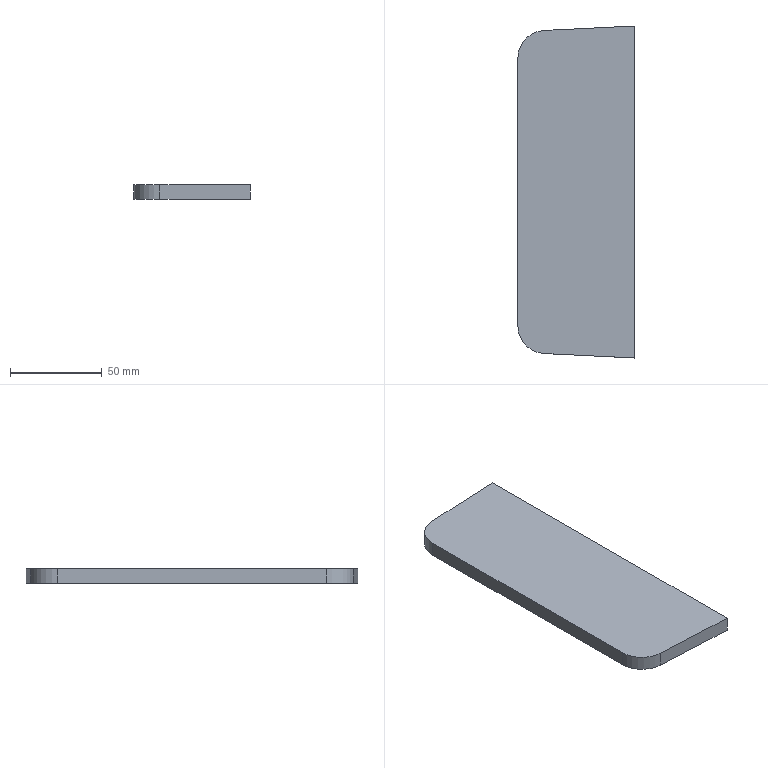Part | SolidWorks | features Extrusion 1 | 1 solid | 8 faces | box 63.5 x 181.351 x 8 mm | volume 89849 mm3 | plane 6 | cylinder 2 | commonest cylinder face diameters 30 x2
STEP:
#1=CARTESIAN_POINT('',(-31.75,-73.268,-4.));
#2=VERTEX_POINT('',#1);
#3=CARTESIAN_POINT('',(-17.488,-88.25,-4.));
#4=VERTEX_POINT('',#3);
#5=CARTESIAN_POINT('',(-16.75,-73.268,-4.));
#6=DIRECTION('',(0.,0.,1.));
#7=DIRECTION('',(1.,0.,0.));
#8=AXIS2_PLACEMENT_3D('',#5,#6,#7);
#9=CIRCLE('',#8,15.);
#10=EDGE_CURVE('',#2,#4,#9,.T.);
#11=ORIENTED_EDGE('',*,*,#10,.T.);
#12=CARTESIAN_POINT('',(-17.488,-88.25,4.));
#13=VERTEX_POINT('',#12);
#14=CARTESIAN_POINT('',(-17.488,-88.25,4.));
#15=DIRECTION('',(0.,0.,-1.));
#16=VECTOR('',#15,1000.);
#17=LINE('',#14,#16);
#18=EDGE_CURVE('',#13,#4,#17,.T.);
#19=ORIENTED_EDGE('',*,*,#18,.F.);
#20=CARTESIAN_POINT('',(-31.75,-73.268,4.));
#21=VERTEX_POINT('',#20);
#22=CARTESIAN_POINT('',(-16.75,-73.268,4.));
#23=DIRECTION('',(0.,0.,1.));
#24=DIRECTION('',(1.,0.,0.));
#25=AXIS2_PLACEMENT_3D('',#22,#23,#24);
#26=CIRCLE('',#25,15.);
#27=EDGE_CURVE('',#21,#13,#26,.T.);
#28=ORIENTED_EDGE('',*,*,#27,.F.);
#29=CARTESIAN_POINT('',(-31.75,-73.268,4.));
#30=DIRECTION('',(0.,0.,-1.));
#31=VECTOR('',#30,1000.);
#32=LINE('',#29,#31);
#33=EDGE_CURVE('',#21,#2,#32,.T.);
#34=ORIENTED_EDGE('',*,*,#33,.T.);
#35=EDGE_LOOP('',(#11,#19,#28,#34));
#36=FACE_OUTER_BOUND('',#35,.T.);
#37=CARTESIAN_POINT('',(-16.75,-73.268,4.));
#38=DIRECTION('',(0.,0.,-1.));
#39=DIRECTION('',(-1.,0.,0.));
#40=AXIS2_PLACEMENT_3D('',#37,#38,#39);
#41=CYLINDRICAL_SURFACE('',#40,15.);
#42=ADVANCED_FACE('',(#36),#41,.T.);
#43=CARTESIAN_POINT('',(31.75,-90.675,-4.));
#44=VERTEX_POINT('',#43);
#45=CARTESIAN_POINT('',(-17.488,-88.25,-4.));
#46=DIRECTION('',(0.9988,-0.0492,0.));
#47=VECTOR('',#46,1000.);
#48=LINE('',#45,#47);
#49=EDGE_CURVE('',#4,#44,#48,.T.);
#50=ORIENTED_EDGE('',*,*,#49,.T.);
#51=CARTESIAN_POINT('',(31.75,-90.675,4.));
#52=VERTEX_POINT('',#51);
#53=CARTESIAN_POINT('',(31.75,-90.675,4.));
#54=DIRECTION('',(0.,0.,-1.));
#55=VECTOR('',#54,1000.);
#56=LINE('',#53,#55);
#57=EDGE_CURVE('',#52,#44,#56,.T.);
#58=ORIENTED_EDGE('',*,*,#57,.F.);
#59=CARTESIAN_POINT('',(-17.488,-88.25,4.));
#60=DIRECTION('',(0.9988,-0.0492,0.));
#61=VECTOR('',#60,1000.);
#62=LINE('',#59,#61);
#63=EDGE_CURVE('',#13,#52,#62,.T.);
#64=ORIENTED_EDGE('',*,*,#63,.F.);
#65=ORIENTED_EDGE('',*,*,#18,.T.);
#66=EDGE_LOOP('',(#50,#58,#64,#65));
#67=FACE_OUTER_BOUND('',#66,.T.);
#68=CARTESIAN_POINT('',(-17.488,-88.25,4.));
#69=DIRECTION('',(0.0492,0.9988,0.));
#70=DIRECTION('',(-0.9988,0.0492,0.));
#71=AXIS2_PLACEMENT_3D('',#68,#69,#70);
#72=PLANE('',#71);
#73=ADVANCED_FACE('',(#67),#72,.F.);
#74=CARTESIAN_POINT('',(31.75,90.675,-4.));
#75=VERTEX_POINT('',#74);
#76=CARTESIAN_POINT('',(31.75,90.675,-4.));
#77=DIRECTION('',(0.,1.,0.));
#78=VECTOR('',#77,1000.);
#79=LINE('',#76,#78);
#80=EDGE_CURVE('',#44,#75,#79,.T.);
#81=ORIENTED_EDGE('',*,*,#80,.T.);
#82=CARTESIAN_POINT('',(31.75,90.675,4.));
#83=VERTEX_POINT('',#82);
#84=CARTESIAN_POINT('',(31.75,90.675,4.));
#85=DIRECTION('',(0.,0.,-1.));
#86=VECTOR('',#85,1000.);
#87=LINE('',#84,#86);
#88=EDGE_CURVE('',#83,#75,#87,.T.);
#89=ORIENTED_EDGE('',*,*,#88,.F.);
#90=CARTESIAN_POINT('',(31.75,90.675,4.));
#91=DIRECTION('',(0.,1.,0.));
#92=VECTOR('',#91,1000.);
#93=LINE('',#90,#92);
#94=EDGE_CURVE('',#52,#83,#93,.T.);
#95=ORIENTED_EDGE('',*,*,#94,.F.);
#96=ORIENTED_EDGE('',*,*,#57,.T.);
#97=EDGE_LOOP('',(#81,#89,#95,#96));
#98=FACE_OUTER_BOUND('',#97,.T.);
#99=CARTESIAN_POINT('',(31.75,90.675,4.));
#100=DIRECTION('',(-1.,0.,0.));
#101=DIRECTION('',(0.,0.,1.));
#102=AXIS2_PLACEMENT_3D('',#99,#100,#101);
#103=PLANE('',#102);
#104=ADVANCED_FACE('',(#98),#103,.F.);
#105=CARTESIAN_POINT('',(-17.488,88.25,-4.));
#106=VERTEX_POINT('',#105);
#107=CARTESIAN_POINT('',(-17.488,88.25,-4.));
#108=DIRECTION('',(-0.9988,-0.0492,0.));
#109=VECTOR('',#108,1000.);
#110=LINE('',#107,#109);
#111=EDGE_CURVE('',#75,#106,#110,.T.);
#112=ORIENTED_EDGE('',*,*,#111,.T.);
#113=CARTESIAN_POINT('',(-17.488,88.25,4.));
#114=VERTEX_POINT('',#113);
#115=CARTESIAN_POINT('',(-17.488,88.25,4.));
#116=DIRECTION('',(0.,0.,-1.));
#117=VECTOR('',#116,1000.);
#118=LINE('',#115,#117);
#119=EDGE_CURVE('',#114,#106,#118,.T.);
#120=ORIENTED_EDGE('',*,*,#119,.F.);
#121=CARTESIAN_POINT('',(-17.488,88.25,4.));
#122=DIRECTION('',(-0.9988,-0.0492,0.));
#123=VECTOR('',#122,1000.);
#124=LINE('',#121,#123);
#125=EDGE_CURVE('',#83,#114,#124,.T.);
#126=ORIENTED_EDGE('',*,*,#125,.F.);
#127=ORIENTED_EDGE('',*,*,#88,.T.);
#128=EDGE_LOOP('',(#112,#120,#126,#127));
#129=FACE_OUTER_BOUND('',#128,.T.);
#130=CARTESIAN_POINT('',(-17.488,88.25,4.));
#131=DIRECTION('',(0.0492,-0.9988,0.));
#132=DIRECTION('',(0.9988,0.0492,0.));
#133=AXIS2_PLACEMENT_3D('',#130,#131,#132);
#134=PLANE('',#133);
#135=ADVANCED_FACE('',(#129),#134,.F.);
#136=CARTESIAN_POINT('',(-31.75,73.268,-4.));
#137=VERTEX_POINT('',#136);
#138=CARTESIAN_POINT('',(-16.75,73.268,-4.));
#139=DIRECTION('',(0.,0.,1.));
#140=DIRECTION('',(-1.,0.,0.));
#141=AXIS2_PLACEMENT_3D('',#138,#139,#140);
#142=CIRCLE('',#141,15.);
#143=EDGE_CURVE('',#106,#137,#142,.T.);
#144=ORIENTED_EDGE('',*,*,#143,.T.);
#145=CARTESIAN_POINT('',(-31.75,73.268,4.));
#146=VERTEX_POINT('',#145);
#147=CARTESIAN_POINT('',(-31.75,73.268,4.));
#148=DIRECTION('',(0.,0.,-1.));
#149=VECTOR('',#148,1000.);
#150=LINE('',#147,#149);
#151=EDGE_CURVE('',#146,#137,#150,.T.);
#152=ORIENTED_EDGE('',*,*,#151,.F.);
#153=CARTESIAN_POINT('',(-16.75,73.268,4.));
#154=DIRECTION('',(0.,0.,1.));
#155=DIRECTION('',(-1.,0.,0.));
#156=AXIS2_PLACEMENT_3D('',#153,#154,#155);
#157=CIRCLE('',#156,15.);
#158=EDGE_CURVE('',#114,#146,#157,.T.);
#159=ORIENTED_EDGE('',*,*,#158,.F.);
#160=ORIENTED_EDGE('',*,*,#119,.T.);
#161=EDGE_LOOP('',(#144,#152,#159,#160));
#162=FACE_OUTER_BOUND('',#161,.T.);
#163=CARTESIAN_POINT('',(-16.75,73.268,4.));
#164=DIRECTION('',(0.,0.,-1.));
#165=DIRECTION('',(-1.,0.,0.));
#166=AXIS2_PLACEMENT_3D('',#163,#164,#165);
#167=CYLINDRICAL_SURFACE('',#166,15.);
#168=ADVANCED_FACE('',(#162),#167,.T.);
#169=CARTESIAN_POINT('',(-31.75,73.268,-4.));
#170=DIRECTION('',(0.,-1.,0.));
#171=VECTOR('',#170,1000.);
#172=LINE('',#169,#171);
#173=EDGE_CURVE('',#137,#2,#172,.T.);
#174=ORIENTED_EDGE('',*,*,#173,.T.);
#175=ORIENTED_EDGE('',*,*,#33,.F.);
#176=CARTESIAN_POINT('',(-31.75,73.268,4.));
#177=DIRECTION('',(0.,-1.,0.));
#178=VECTOR('',#177,1000.);
#179=LINE('',#176,#178);
#180=EDGE_CURVE('',#146,#21,#179,.T.);
#181=ORIENTED_EDGE('',*,*,#180,.F.);
#182=ORIENTED_EDGE('',*,*,#151,.T.);
#183=EDGE_LOOP('',(#174,#175,#181,#182));
#184=FACE_OUTER_BOUND('',#183,.T.);
#185=CARTESIAN_POINT('',(-31.75,73.268,4.));
#186=DIRECTION('',(1.,0.,0.));
#187=DIRECTION('',(0.,0.,-1.));
#188=AXIS2_PLACEMENT_3D('',#185,#186,#187);
#189=PLANE('',#188);
#190=ADVANCED_FACE('',(#184),#189,.F.);
#191=ORIENTED_EDGE('',*,*,#27,.T.);
#192=ORIENTED_EDGE('',*,*,#63,.T.);
#193=ORIENTED_EDGE('',*,*,#94,.T.);
#194=ORIENTED_EDGE('',*,*,#125,.T.);
#195=ORIENTED_EDGE('',*,*,#158,.T.);
#196=ORIENTED_EDGE('',*,*,#180,.T.);
#197=EDGE_LOOP('',(#191,#192,#193,#194,#195,#196));
#198=FACE_OUTER_BOUND('',#197,.T.);
#199=CARTESIAN_POINT('',(-16.75,-73.268,4.));
#200=DIRECTION('',(0.,0.,1.));
#201=DIRECTION('',(1.,0.,0.));
#202=AXIS2_PLACEMENT_3D('',#199,#200,#201);
#203=PLANE('',#202);
#204=ADVANCED_FACE('',(#198),#203,.T.);
#205=ORIENTED_EDGE('',*,*,#10,.F.);
#206=ORIENTED_EDGE('',*,*,#173,.F.);
#207=ORIENTED_EDGE('',*,*,#143,.F.);
#208=ORIENTED_EDGE('',*,*,#111,.F.);
#209=ORIENTED_EDGE('',*,*,#80,.F.);
#210=ORIENTED_EDGE('',*,*,#49,.F.);
#211=EDGE_LOOP('',(#205,#206,#207,#208,#209,#210));
#212=FACE_OUTER_BOUND('',#211,.T.);
#213=CARTESIAN_POINT('',(-16.75,-73.268,-4.));
#214=DIRECTION('',(0.,0.,1.));
#215=DIRECTION('',(1.,0.,0.));
#216=AXIS2_PLACEMENT_3D('',#213,#214,#215);
#217=PLANE('',#216);
#218=ADVANCED_FACE('',(#212),#217,.F.);
#219=CLOSED_SHELL('',(#42,#73,#104,#135,#168,#190,#204,#218));
#220=MANIFOLD_SOLID_BREP('',#219);
#221=CARTESIAN_POINT('',(0.,0.,0.));
#222=DIRECTION('',(0.,0.,1.));
#223=DIRECTION('',(1.,0.,0.));
#224=AXIS2_PLACEMENT_3D('',#221,#222,#223);
#225=(LENGTH_UNIT()NAMED_UNIT(*)SI_UNIT(.MILLI.,.METRE.));
#226=UNCERTAINTY_MEASURE_WITH_UNIT(LENGTH_MEASURE(0.00001),#225,'','');
#227=(NAMED_UNIT(*)PLANE_ANGLE_UNIT()SI_UNIT($,.RADIAN.));
#228=(NAMED_UNIT(*)SI_UNIT($,.STERADIAN.)SOLID_ANGLE_UNIT());
#229=(GEOMETRIC_REPRESENTATION_CONTEXT(3)GLOBAL_UNCERTAINTY_ASSIGNED_CONTEXT((#226))GLOBAL_UNIT_ASSIGNED_CONTEXT((#225,#227,#228))REPRESENTATION_CONTEXT('',''));
#230=ADVANCED_BREP_SHAPE_REPRESENTATION('',(#220,#224),#229);